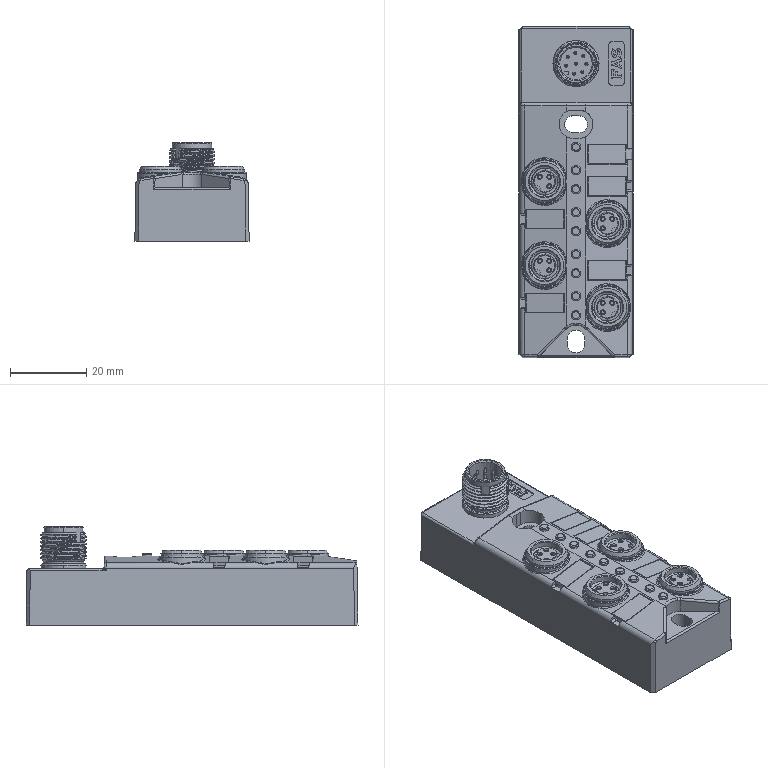Part | STEP file | 17 solids | 2022 faces | box 29.939 x 86.939 x 25.75 mm | volume 39070 mm3 | plane 702 | cylinder 589 | cone 405 | spline 324 | torus 2 | commonest cylinder face diameters 0.8 x106 1.6 x73 1 x60 1.2 x47 8.1 x40 1.35 x36